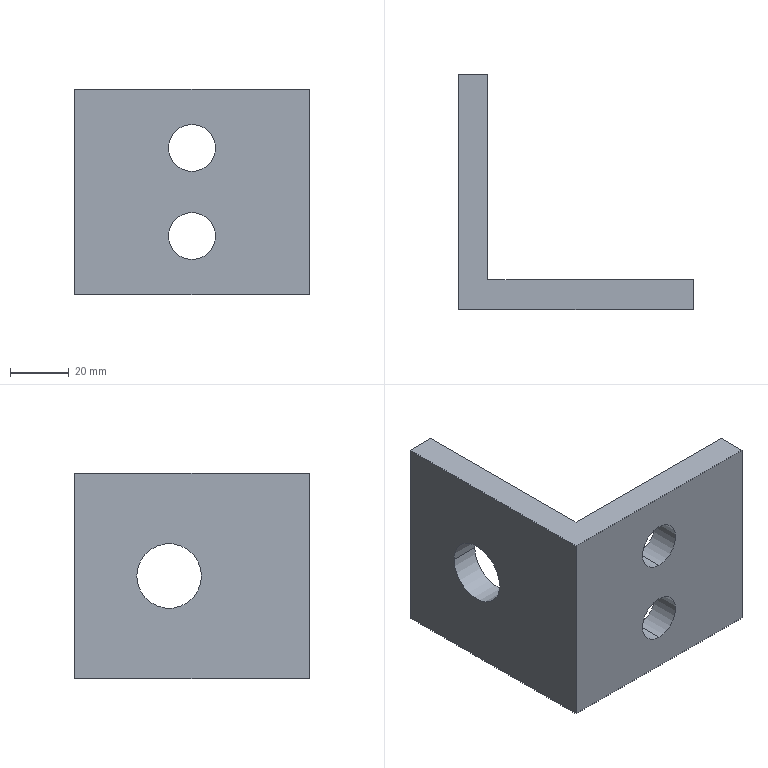Part | SolidWorks | features ICE 2, Extrusion 1 | 1 solid | 14 faces | box 80 x 80 x 70 mm | volume 97177 mm3 | plane 8 | cylinder 6 | commonest cylinder face diameters 16 x4 22 x2
STEP:
#1=CARTESIAN_POINT('',(0.,36.792,35.));
#2=VERTEX_POINT('',#1);
#3=CARTESIAN_POINT('',(0.,58.792,35.));
#4=VERTEX_POINT('',#3);
#5=CARTESIAN_POINT('',(0.,47.792,35.));
#6=DIRECTION('',(1.,0.,0.));
#7=DIRECTION('',(0.,0.,-1.));
#8=AXIS2_PLACEMENT_3D('',#5,#6,#7);
#9=CIRCLE('',#8,11.);
#10=EDGE_CURVE('',#2,#4,#9,.T.);
#11=ORIENTED_EDGE('',*,*,#10,.F.);
#12=CARTESIAN_POINT('',(10.,36.792,35.));
#13=VERTEX_POINT('',#12);
#14=CARTESIAN_POINT('',(-80.,36.792,35.));
#15=DIRECTION('',(1.,0.,0.));
#16=VECTOR('',#15,1000.);
#17=LINE('',#14,#16);
#18=EDGE_CURVE('',#2,#13,#17,.T.);
#19=ORIENTED_EDGE('',*,*,#18,.T.);
#20=CARTESIAN_POINT('',(10.,58.792,35.));
#21=VERTEX_POINT('',#20);
#22=CARTESIAN_POINT('',(10.,47.792,35.));
#23=DIRECTION('',(1.,0.,0.));
#24=DIRECTION('',(0.,1.,0.));
#25=AXIS2_PLACEMENT_3D('',#22,#23,#24);
#26=CIRCLE('',#25,11.);
#27=EDGE_CURVE('',#13,#21,#26,.T.);
#28=ORIENTED_EDGE('',*,*,#27,.T.);
#29=CARTESIAN_POINT('',(-80.,58.792,35.));
#30=DIRECTION('',(1.,0.,0.));
#31=VECTOR('',#30,1000.);
#32=LINE('',#29,#31);
#33=EDGE_CURVE('',#4,#21,#32,.T.);
#34=ORIENTED_EDGE('',*,*,#33,.F.);
#35=EDGE_LOOP('',(#11,#19,#28,#34));
#36=FACE_OUTER_BOUND('',#35,.T.);
#37=CARTESIAN_POINT('',(-80.,47.792,35.));
#38=DIRECTION('',(1.,0.,0.));
#39=DIRECTION('',(0.,1.,0.));
#40=AXIS2_PLACEMENT_3D('',#37,#38,#39);
#41=CYLINDRICAL_SURFACE('',#40,11.);
#42=ADVANCED_FACE('',(#36),#41,.F.);
#43=CARTESIAN_POINT('',(40.,0.,12.));
#44=VERTEX_POINT('',#43);
#45=CARTESIAN_POINT('',(40.,0.,28.));
#46=VERTEX_POINT('',#45);
#47=CARTESIAN_POINT('',(40.,0.,20.));
#48=DIRECTION('',(0.,1.,0.));
#49=DIRECTION('',(-1.,0.,0.));
#50=AXIS2_PLACEMENT_3D('',#47,#48,#49);
#51=CIRCLE('',#50,8.);
#52=EDGE_CURVE('',#44,#46,#51,.T.);
#53=ORIENTED_EDGE('',*,*,#52,.F.);
#54=CARTESIAN_POINT('',(40.,10.,12.));
#55=VERTEX_POINT('',#54);
#56=CARTESIAN_POINT('',(40.,-80.,12.));
#57=DIRECTION('',(0.,1.,0.));
#58=VECTOR('',#57,1000.);
#59=LINE('',#56,#58);
#60=EDGE_CURVE('',#44,#55,#59,.T.);
#61=ORIENTED_EDGE('',*,*,#60,.T.);
#62=CARTESIAN_POINT('',(40.,10.,28.));
#63=VERTEX_POINT('',#62);
#64=CARTESIAN_POINT('',(40.,10.,20.));
#65=DIRECTION('',(0.,1.,0.));
#66=DIRECTION('',(0.,0.,1.));
#67=AXIS2_PLACEMENT_3D('',#64,#65,#66);
#68=CIRCLE('',#67,8.);
#69=EDGE_CURVE('',#55,#63,#68,.T.);
#70=ORIENTED_EDGE('',*,*,#69,.T.);
#71=CARTESIAN_POINT('',(40.,-80.,28.));
#72=DIRECTION('',(0.,1.,0.));
#73=VECTOR('',#72,1000.);
#74=LINE('',#71,#73);
#75=EDGE_CURVE('',#46,#63,#74,.T.);
#76=ORIENTED_EDGE('',*,*,#75,.F.);
#77=EDGE_LOOP('',(#53,#61,#70,#76));
#78=FACE_OUTER_BOUND('',#77,.T.);
#79=CARTESIAN_POINT('',(40.,-80.,20.));
#80=DIRECTION('',(0.,1.,0.));
#81=DIRECTION('',(0.,0.,1.));
#82=AXIS2_PLACEMENT_3D('',#79,#80,#81);
#83=CYLINDRICAL_SURFACE('',#82,8.);
#84=ADVANCED_FACE('',(#78),#83,.F.);
#85=CARTESIAN_POINT('',(40.,0.,42.));
#86=VERTEX_POINT('',#85);
#87=CARTESIAN_POINT('',(40.,0.,58.));
#88=VERTEX_POINT('',#87);
#89=CARTESIAN_POINT('',(40.,0.,50.));
#90=DIRECTION('',(0.,1.,0.));
#91=DIRECTION('',(-1.,0.,0.));
#92=AXIS2_PLACEMENT_3D('',#89,#90,#91);
#93=CIRCLE('',#92,8.);
#94=EDGE_CURVE('',#86,#88,#93,.T.);
#95=ORIENTED_EDGE('',*,*,#94,.F.);
#96=CARTESIAN_POINT('',(40.,10.,42.));
#97=VERTEX_POINT('',#96);
#98=CARTESIAN_POINT('',(40.,-80.,42.));
#99=DIRECTION('',(0.,1.,0.));
#100=VECTOR('',#99,1000.);
#101=LINE('',#98,#100);
#102=EDGE_CURVE('',#86,#97,#101,.T.);
#103=ORIENTED_EDGE('',*,*,#102,.T.);
#104=CARTESIAN_POINT('',(40.,10.,58.));
#105=VERTEX_POINT('',#104);
#106=CARTESIAN_POINT('',(40.,10.,50.));
#107=DIRECTION('',(0.,1.,0.));
#108=DIRECTION('',(0.,0.,1.));
#109=AXIS2_PLACEMENT_3D('',#106,#107,#108);
#110=CIRCLE('',#109,8.);
#111=EDGE_CURVE('',#97,#105,#110,.T.);
#112=ORIENTED_EDGE('',*,*,#111,.T.);
#113=CARTESIAN_POINT('',(40.,-80.,58.));
#114=DIRECTION('',(0.,1.,0.));
#115=VECTOR('',#114,1000.);
#116=LINE('',#113,#115);
#117=EDGE_CURVE('',#88,#105,#116,.T.);
#118=ORIENTED_EDGE('',*,*,#117,.F.);
#119=EDGE_LOOP('',(#95,#103,#112,#118));
#120=FACE_OUTER_BOUND('',#119,.T.);
#121=CARTESIAN_POINT('',(40.,-80.,50.));
#122=DIRECTION('',(0.,1.,0.));
#123=DIRECTION('',(0.,0.,1.));
#124=AXIS2_PLACEMENT_3D('',#121,#122,#123);
#125=CYLINDRICAL_SURFACE('',#124,8.);
#126=ADVANCED_FACE('',(#120),#125,.F.);
#127=CARTESIAN_POINT('',(40.,0.,20.));
#128=DIRECTION('',(0.,1.,0.));
#129=DIRECTION('',(-1.,0.,0.));
#130=AXIS2_PLACEMENT_3D('',#127,#128,#129);
#131=CIRCLE('',#130,8.);
#132=EDGE_CURVE('',#46,#44,#131,.T.);
#133=ORIENTED_EDGE('',*,*,#132,.T.);
#134=ORIENTED_EDGE('',*,*,#52,.T.);
#135=EDGE_LOOP('',(#133,#134));
#136=FACE_BOUND('',#135,.T.);
#137=CARTESIAN_POINT('',(40.,0.,50.));
#138=DIRECTION('',(0.,1.,0.));
#139=DIRECTION('',(-1.,0.,0.));
#140=AXIS2_PLACEMENT_3D('',#137,#138,#139);
#141=CIRCLE('',#140,8.);
#142=EDGE_CURVE('',#88,#86,#141,.T.);
#143=ORIENTED_EDGE('',*,*,#142,.T.);
#144=ORIENTED_EDGE('',*,*,#94,.T.);
#145=EDGE_LOOP('',(#143,#144));
#146=FACE_BOUND('',#145,.T.);
#147=CARTESIAN_POINT('',(0.,0.,0.));
#148=VERTEX_POINT('',#147);
#149=CARTESIAN_POINT('',(80.,0.,0.));
#150=VERTEX_POINT('',#149);
#151=CARTESIAN_POINT('',(80.,0.,0.));
#152=DIRECTION('',(1.,0.,0.));
#153=VECTOR('',#152,1000.);
#154=LINE('',#151,#153);
#155=EDGE_CURVE('',#148,#150,#154,.T.);
#156=ORIENTED_EDGE('',*,*,#155,.T.);
#157=CARTESIAN_POINT('',(80.,0.,70.));
#158=VERTEX_POINT('',#157);
#159=CARTESIAN_POINT('',(80.,0.,70.));
#160=DIRECTION('',(0.,0.,-1.));
#161=VECTOR('',#160,1000.);
#162=LINE('',#159,#161);
#163=EDGE_CURVE('',#158,#150,#162,.T.);
#164=ORIENTED_EDGE('',*,*,#163,.F.);
#165=CARTESIAN_POINT('',(0.,0.,70.));
#166=VERTEX_POINT('',#165);
#167=CARTESIAN_POINT('',(80.,0.,70.));
#168=DIRECTION('',(1.,0.,0.));
#169=VECTOR('',#168,1000.);
#170=LINE('',#167,#169);
#171=EDGE_CURVE('',#166,#158,#170,.T.);
#172=ORIENTED_EDGE('',*,*,#171,.F.);
#173=CARTESIAN_POINT('',(0.,0.,70.));
#174=DIRECTION('',(0.,0.,-1.));
#175=VECTOR('',#174,1000.);
#176=LINE('',#173,#175);
#177=EDGE_CURVE('',#166,#148,#176,.T.);
#178=ORIENTED_EDGE('',*,*,#177,.T.);
#179=EDGE_LOOP('',(#156,#164,#172,#178));
#180=FACE_OUTER_BOUND('',#179,.T.);
#181=CARTESIAN_POINT('',(80.,0.,70.));
#182=DIRECTION('',(0.,1.,0.));
#183=DIRECTION('',(-1.,0.,0.));
#184=AXIS2_PLACEMENT_3D('',#181,#182,#183);
#185=PLANE('',#184);
#186=ADVANCED_FACE('',(#136,#146,#180),#185,.F.);
#187=CARTESIAN_POINT('',(80.,10.,0.));
#188=VERTEX_POINT('',#187);
#189=CARTESIAN_POINT('',(80.,10.,0.));
#190=DIRECTION('',(0.,1.,0.));
#191=VECTOR('',#190,1000.);
#192=LINE('',#189,#191);
#193=EDGE_CURVE('',#150,#188,#192,.T.);
#194=ORIENTED_EDGE('',*,*,#193,.T.);
#195=CARTESIAN_POINT('',(80.,10.,70.));
#196=VERTEX_POINT('',#195);
#197=CARTESIAN_POINT('',(80.,10.,70.));
#198=DIRECTION('',(0.,0.,-1.));
#199=VECTOR('',#198,1000.);
#200=LINE('',#197,#199);
#201=EDGE_CURVE('',#196,#188,#200,.T.);
#202=ORIENTED_EDGE('',*,*,#201,.F.);
#203=CARTESIAN_POINT('',(80.,10.,70.));
#204=DIRECTION('',(0.,1.,0.));
#205=VECTOR('',#204,1000.);
#206=LINE('',#203,#205);
#207=EDGE_CURVE('',#158,#196,#206,.T.);
#208=ORIENTED_EDGE('',*,*,#207,.F.);
#209=ORIENTED_EDGE('',*,*,#163,.T.);
#210=EDGE_LOOP('',(#194,#202,#208,#209));
#211=FACE_OUTER_BOUND('',#210,.T.);
#212=CARTESIAN_POINT('',(80.,10.,70.));
#213=DIRECTION('',(-1.,0.,0.));
#214=DIRECTION('',(0.,0.,1.));
#215=AXIS2_PLACEMENT_3D('',#212,#213,#214);
#216=PLANE('',#215);
#217=ADVANCED_FACE('',(#211),#216,.F.);
#218=CARTESIAN_POINT('',(40.,10.,20.));
#219=DIRECTION('',(0.,1.,0.));
#220=DIRECTION('',(0.,0.,1.));
#221=AXIS2_PLACEMENT_3D('',#218,#219,#220);
#222=CIRCLE('',#221,8.);
#223=EDGE_CURVE('',#63,#55,#222,.T.);
#224=ORIENTED_EDGE('',*,*,#223,.F.);
#225=ORIENTED_EDGE('',*,*,#69,.F.);
#226=EDGE_LOOP('',(#224,#225));
#227=FACE_BOUND('',#226,.T.);
#228=CARTESIAN_POINT('',(40.,10.,50.));
#229=DIRECTION('',(0.,1.,0.));
#230=DIRECTION('',(0.,0.,1.));
#231=AXIS2_PLACEMENT_3D('',#228,#229,#230);
#232=CIRCLE('',#231,8.);
#233=EDGE_CURVE('',#105,#97,#232,.T.);
#234=ORIENTED_EDGE('',*,*,#233,.F.);
#235=ORIENTED_EDGE('',*,*,#111,.F.);
#236=EDGE_LOOP('',(#234,#235));
#237=FACE_BOUND('',#236,.T.);
#238=CARTESIAN_POINT('',(10.,10.,0.));
#239=VERTEX_POINT('',#238);
#240=CARTESIAN_POINT('',(10.,10.,0.));
#241=DIRECTION('',(-1.,0.,0.));
#242=VECTOR('',#241,1000.);
#243=LINE('',#240,#242);
#244=EDGE_CURVE('',#188,#239,#243,.T.);
#245=ORIENTED_EDGE('',*,*,#244,.T.);
#246=CARTESIAN_POINT('',(10.,10.,70.));
#247=VERTEX_POINT('',#246);
#248=CARTESIAN_POINT('',(10.,10.,70.));
#249=DIRECTION('',(0.,0.,-1.));
#250=VECTOR('',#249,1000.);
#251=LINE('',#248,#250);
#252=EDGE_CURVE('',#247,#239,#251,.T.);
#253=ORIENTED_EDGE('',*,*,#252,.F.);
#254=CARTESIAN_POINT('',(10.,10.,70.));
#255=DIRECTION('',(-1.,0.,0.));
#256=VECTOR('',#255,1000.);
#257=LINE('',#254,#256);
#258=EDGE_CURVE('',#196,#247,#257,.T.);
#259=ORIENTED_EDGE('',*,*,#258,.F.);
#260=ORIENTED_EDGE('',*,*,#201,.T.);
#261=EDGE_LOOP('',(#245,#253,#259,#260));
#262=FACE_OUTER_BOUND('',#261,.T.);
#263=CARTESIAN_POINT('',(10.,10.,70.));
#264=DIRECTION('',(0.,-1.,0.));
#265=DIRECTION('',(0.,0.,-1.));
#266=AXIS2_PLACEMENT_3D('',#263,#264,#265);
#267=PLANE('',#266);
#268=ADVANCED_FACE('',(#227,#237,#262),#267,.F.);
#269=CARTESIAN_POINT('',(10.,47.792,35.));
#270=DIRECTION('',(1.,0.,0.));
#271=DIRECTION('',(0.,1.,0.));
#272=AXIS2_PLACEMENT_3D('',#269,#270,#271);
#273=CIRCLE('',#272,11.);
#274=EDGE_CURVE('',#21,#13,#273,.T.);
#275=ORIENTED_EDGE('',*,*,#274,.F.);
#276=ORIENTED_EDGE('',*,*,#27,.F.);
#277=EDGE_LOOP('',(#275,#276));
#278=FACE_BOUND('',#277,.T.);
#279=CARTESIAN_POINT('',(10.,80.,0.));
#280=VERTEX_POINT('',#279);
#281=CARTESIAN_POINT('',(10.,80.,0.));
#282=DIRECTION('',(0.,1.,0.));
#283=VECTOR('',#282,1000.);
#284=LINE('',#281,#283);
#285=EDGE_CURVE('',#239,#280,#284,.T.);
#286=ORIENTED_EDGE('',*,*,#285,.T.);
#287=CARTESIAN_POINT('',(10.,80.,70.));
#288=VERTEX_POINT('',#287);
#289=CARTESIAN_POINT('',(10.,80.,70.));
#290=DIRECTION('',(0.,0.,-1.));
#291=VECTOR('',#290,1000.);
#292=LINE('',#289,#291);
#293=EDGE_CURVE('',#288,#280,#292,.T.);
#294=ORIENTED_EDGE('',*,*,#293,.F.);
#295=CARTESIAN_POINT('',(10.,80.,70.));
#296=DIRECTION('',(0.,1.,0.));
#297=VECTOR('',#296,1000.);
#298=LINE('',#295,#297);
#299=EDGE_CURVE('',#247,#288,#298,.T.);
#300=ORIENTED_EDGE('',*,*,#299,.F.);
#301=ORIENTED_EDGE('',*,*,#252,.T.);
#302=EDGE_LOOP('',(#286,#294,#300,#301));
#303=FACE_OUTER_BOUND('',#302,.T.);
#304=CARTESIAN_POINT('',(10.,80.,70.));
#305=DIRECTION('',(-1.,0.,0.));
#306=DIRECTION('',(0.,-1.,0.));
#307=AXIS2_PLACEMENT_3D('',#304,#305,#306);
#308=PLANE('',#307);
#309=ADVANCED_FACE('',(#278,#303),#308,.F.);
#310=CARTESIAN_POINT('',(0.,80.,0.));
#311=VERTEX_POINT('',#310);
#312=CARTESIAN_POINT('',(0.,80.,0.));
#313=DIRECTION('',(-1.,0.,0.));
#314=VECTOR('',#313,1000.);
#315=LINE('',#312,#314);
#316=EDGE_CURVE('',#280,#311,#315,.T.);
#317=ORIENTED_EDGE('',*,*,#316,.T.);
#318=CARTESIAN_POINT('',(0.,80.,70.));
#319=VERTEX_POINT('',#318);
#320=CARTESIAN_POINT('',(0.,80.,70.));
#321=DIRECTION('',(0.,0.,-1.));
#322=VECTOR('',#321,1000.);
#323=LINE('',#320,#322);
#324=EDGE_CURVE('',#319,#311,#323,.T.);
#325=ORIENTED_EDGE('',*,*,#324,.F.);
#326=CARTESIAN_POINT('',(0.,80.,70.));
#327=DIRECTION('',(-1.,0.,0.));
#328=VECTOR('',#327,1000.);
#329=LINE('',#326,#328);
#330=EDGE_CURVE('',#288,#319,#329,.T.);
#331=ORIENTED_EDGE('',*,*,#330,.F.);
#332=ORIENTED_EDGE('',*,*,#293,.T.);
#333=EDGE_LOOP('',(#317,#325,#331,#332));
#334=FACE_OUTER_BOUND('',#333,.T.);
#335=CARTESIAN_POINT('',(0.,80.,70.));
#336=DIRECTION('',(0.,-1.,0.));
#337=DIRECTION('',(0.,0.,-1.));
#338=AXIS2_PLACEMENT_3D('',#335,#336,#337);
#339=PLANE('',#338);
#340=ADVANCED_FACE('',(#334),#339,.F.);
#341=CARTESIAN_POINT('',(0.,47.792,35.));
#342=DIRECTION('',(1.,0.,0.));
#343=DIRECTION('',(0.,0.,-1.));
#344=AXIS2_PLACEMENT_3D('',#341,#342,#343);
#345=CIRCLE('',#344,11.);
#346=EDGE_CURVE('',#4,#2,#345,.T.);
#347=ORIENTED_EDGE('',*,*,#346,.T.);
#348=ORIENTED_EDGE('',*,*,#10,.T.);
#349=EDGE_LOOP('',(#347,#348));
#350=FACE_BOUND('',#349,.T.);
#351=CARTESIAN_POINT('',(0.,0.,0.));
#352=DIRECTION('',(0.,-1.,0.));
#353=VECTOR('',#352,1000.);
#354=LINE('',#351,#353);
#355=EDGE_CURVE('',#311,#148,#354,.T.);
#356=ORIENTED_EDGE('',*,*,#355,.T.);
#357=ORIENTED_EDGE('',*,*,#177,.F.);
#358=CARTESIAN_POINT('',(0.,0.,70.));
#359=DIRECTION('',(0.,-1.,0.));
#360=VECTOR('',#359,1000.);
#361=LINE('',#358,#360);
#362=EDGE_CURVE('',#319,#166,#361,.T.);
#363=ORIENTED_EDGE('',*,*,#362,.F.);
#364=ORIENTED_EDGE('',*,*,#324,.T.);
#365=EDGE_LOOP('',(#356,#357,#363,#364));
#366=FACE_OUTER_BOUND('',#365,.T.);
#367=CARTESIAN_POINT('',(0.,0.,70.));
#368=DIRECTION('',(1.,0.,0.));
#369=DIRECTION('',(0.,0.,-1.));
#370=AXIS2_PLACEMENT_3D('',#367,#368,#369);
#371=PLANE('',#370);
#372=ADVANCED_FACE('',(#350,#366),#371,.F.);
#373=ORIENTED_EDGE('',*,*,#171,.T.);
#374=ORIENTED_EDGE('',*,*,#207,.T.);
#375=ORIENTED_EDGE('',*,*,#258,.T.);
#376=ORIENTED_EDGE('',*,*,#299,.T.);
#377=ORIENTED_EDGE('',*,*,#330,.T.);
#378=ORIENTED_EDGE('',*,*,#362,.T.);
#379=EDGE_LOOP('',(#373,#374,#375,#376,#377,#378));
#380=FACE_OUTER_BOUND('',#379,.T.);
#381=CARTESIAN_POINT('',(0.,0.,70.));
#382=DIRECTION('',(0.,0.,-1.));
#383=DIRECTION('',(-1.,0.,0.));
#384=AXIS2_PLACEMENT_3D('',#381,#382,#383);
#385=PLANE('',#384);
#386=ADVANCED_FACE('',(#380),#385,.F.);
#387=ORIENTED_EDGE('',*,*,#155,.F.);
#388=ORIENTED_EDGE('',*,*,#355,.F.);
#389=ORIENTED_EDGE('',*,*,#316,.F.);
#390=ORIENTED_EDGE('',*,*,#285,.F.);
#391=ORIENTED_EDGE('',*,*,#244,.F.);
#392=ORIENTED_EDGE('',*,*,#193,.F.);
#393=EDGE_LOOP('',(#387,#388,#389,#390,#391,#392));
#394=FACE_OUTER_BOUND('',#393,.T.);
#395=CARTESIAN_POINT('',(0.,0.,0.));
#396=DIRECTION('',(0.,0.,-1.));
#397=DIRECTION('',(-1.,0.,0.));
#398=AXIS2_PLACEMENT_3D('',#395,#396,#397);
#399=PLANE('',#398);
#400=ADVANCED_FACE('',(#394),#399,.T.);
#401=ORIENTED_EDGE('',*,*,#102,.F.);
#402=ORIENTED_EDGE('',*,*,#142,.F.);
#403=ORIENTED_EDGE('',*,*,#117,.T.);
#404=ORIENTED_EDGE('',*,*,#233,.T.);
#405=EDGE_LOOP('',(#401,#402,#403,#404));
#406=FACE_OUTER_BOUND('',#405,.T.);
#407=CARTESIAN_POINT('',(40.,-80.,50.));
#408=DIRECTION('',(0.,1.,0.));
#409=DIRECTION('',(0.,0.,1.));
#410=AXIS2_PLACEMENT_3D('',#407,#408,#409);
#411=CYLINDRICAL_SURFACE('',#410,8.);
#412=ADVANCED_FACE('',(#406),#411,.F.);
#413=ORIENTED_EDGE('',*,*,#60,.F.);
#414=ORIENTED_EDGE('',*,*,#132,.F.);
#415=ORIENTED_EDGE('',*,*,#75,.T.);
#416=ORIENTED_EDGE('',*,*,#223,.T.);
#417=EDGE_LOOP('',(#413,#414,#415,#416));
#418=FACE_OUTER_BOUND('',#417,.T.);
#419=CARTESIAN_POINT('',(40.,-80.,20.));
#420=DIRECTION('',(0.,1.,0.));
#421=DIRECTION('',(0.,0.,1.));
#422=AXIS2_PLACEMENT_3D('',#419,#420,#421);
#423=CYLINDRICAL_SURFACE('',#422,8.);
#424=ADVANCED_FACE('',(#418),#423,.F.);
#425=ORIENTED_EDGE('',*,*,#18,.F.);
#426=ORIENTED_EDGE('',*,*,#346,.F.);
#427=ORIENTED_EDGE('',*,*,#33,.T.);
#428=ORIENTED_EDGE('',*,*,#274,.T.);
#429=EDGE_LOOP('',(#425,#426,#427,#428));
#430=FACE_OUTER_BOUND('',#429,.T.);
#431=CARTESIAN_POINT('',(-80.,47.792,35.));
#432=DIRECTION('',(1.,0.,0.));
#433=DIRECTION('',(0.,1.,0.));
#434=AXIS2_PLACEMENT_3D('',#431,#432,#433);
#435=CYLINDRICAL_SURFACE('',#434,11.);
#436=ADVANCED_FACE('',(#430),#435,.F.);
#437=CLOSED_SHELL('',(#42,#84,#126,#186,#217,#268,#309,#340,#372,#386,#400,#412,#424,#436));
#438=MANIFOLD_SOLID_BREP('',#437);
#439=CARTESIAN_POINT('',(0.,0.,0.));
#440=DIRECTION('',(0.,0.,1.));
#441=DIRECTION('',(1.,0.,0.));
#442=AXIS2_PLACEMENT_3D('',#439,#440,#441);
#443=(LENGTH_UNIT()NAMED_UNIT(*)SI_UNIT(.MILLI.,.METRE.));
#444=UNCERTAINTY_MEASURE_WITH_UNIT(LENGTH_MEASURE(0.00001),#443,'','');
#445=(NAMED_UNIT(*)PLANE_ANGLE_UNIT()SI_UNIT($,.RADIAN.));
#446=(NAMED_UNIT(*)SI_UNIT($,.STERADIAN.)SOLID_ANGLE_UNIT());
#447=(GEOMETRIC_REPRESENTATION_CONTEXT(3)GLOBAL_UNCERTAINTY_ASSIGNED_CONTEXT((#444))GLOBAL_UNIT_ASSIGNED_CONTEXT((#443,#445,#446))REPRESENTATION_CONTEXT('',''));
#448=ADVANCED_BREP_SHAPE_REPRESENTATION('',(#438,#442),#447);